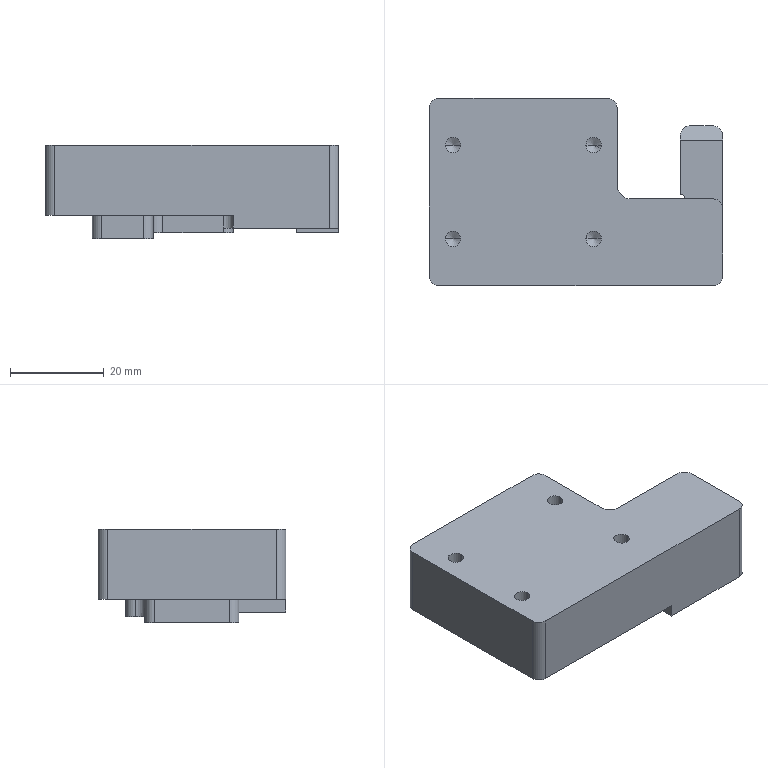Part | STEP file | 04-14 pre-press block | 1 solid | 60 faces | box 62.5 x 40 x 20 mm | volume 33897 mm3 | cylinder 26 | plane 26 | cone 8 | commonest cylinder face diameters 4 x16 3.3 x8 2 x1 6 x1